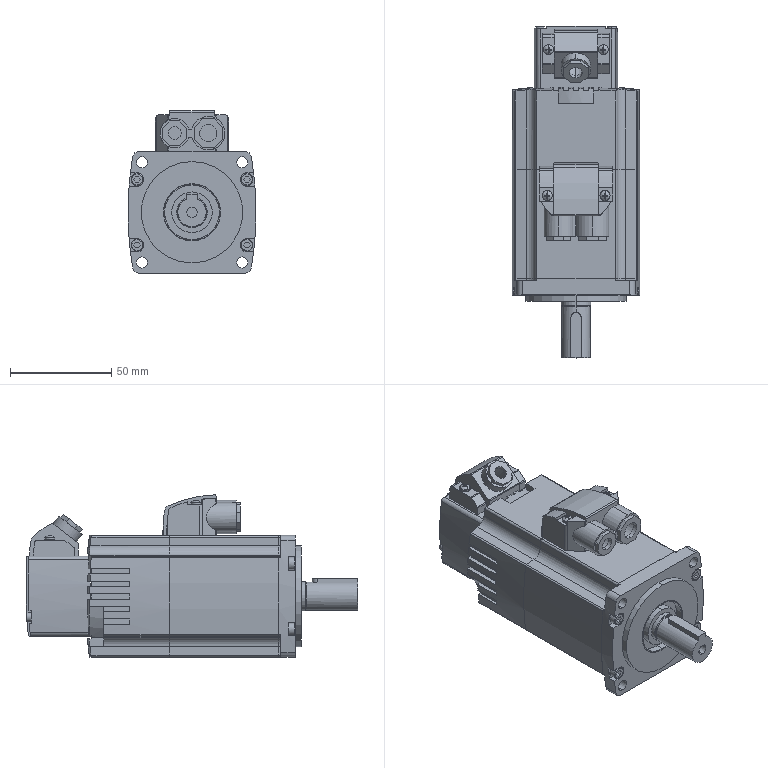Part | SolidWorks | features BaseBody 8 | 8 solids | 759 faces | box 63.062 x 163.688 x 80 mm | volume 352083 mm3 | plane 452 | cylinder 253 | spline 54 | commonest cylinder face diameters 2 x24 1.2 x23 9.4 x12 5 x11 6 x9 2.8 x8